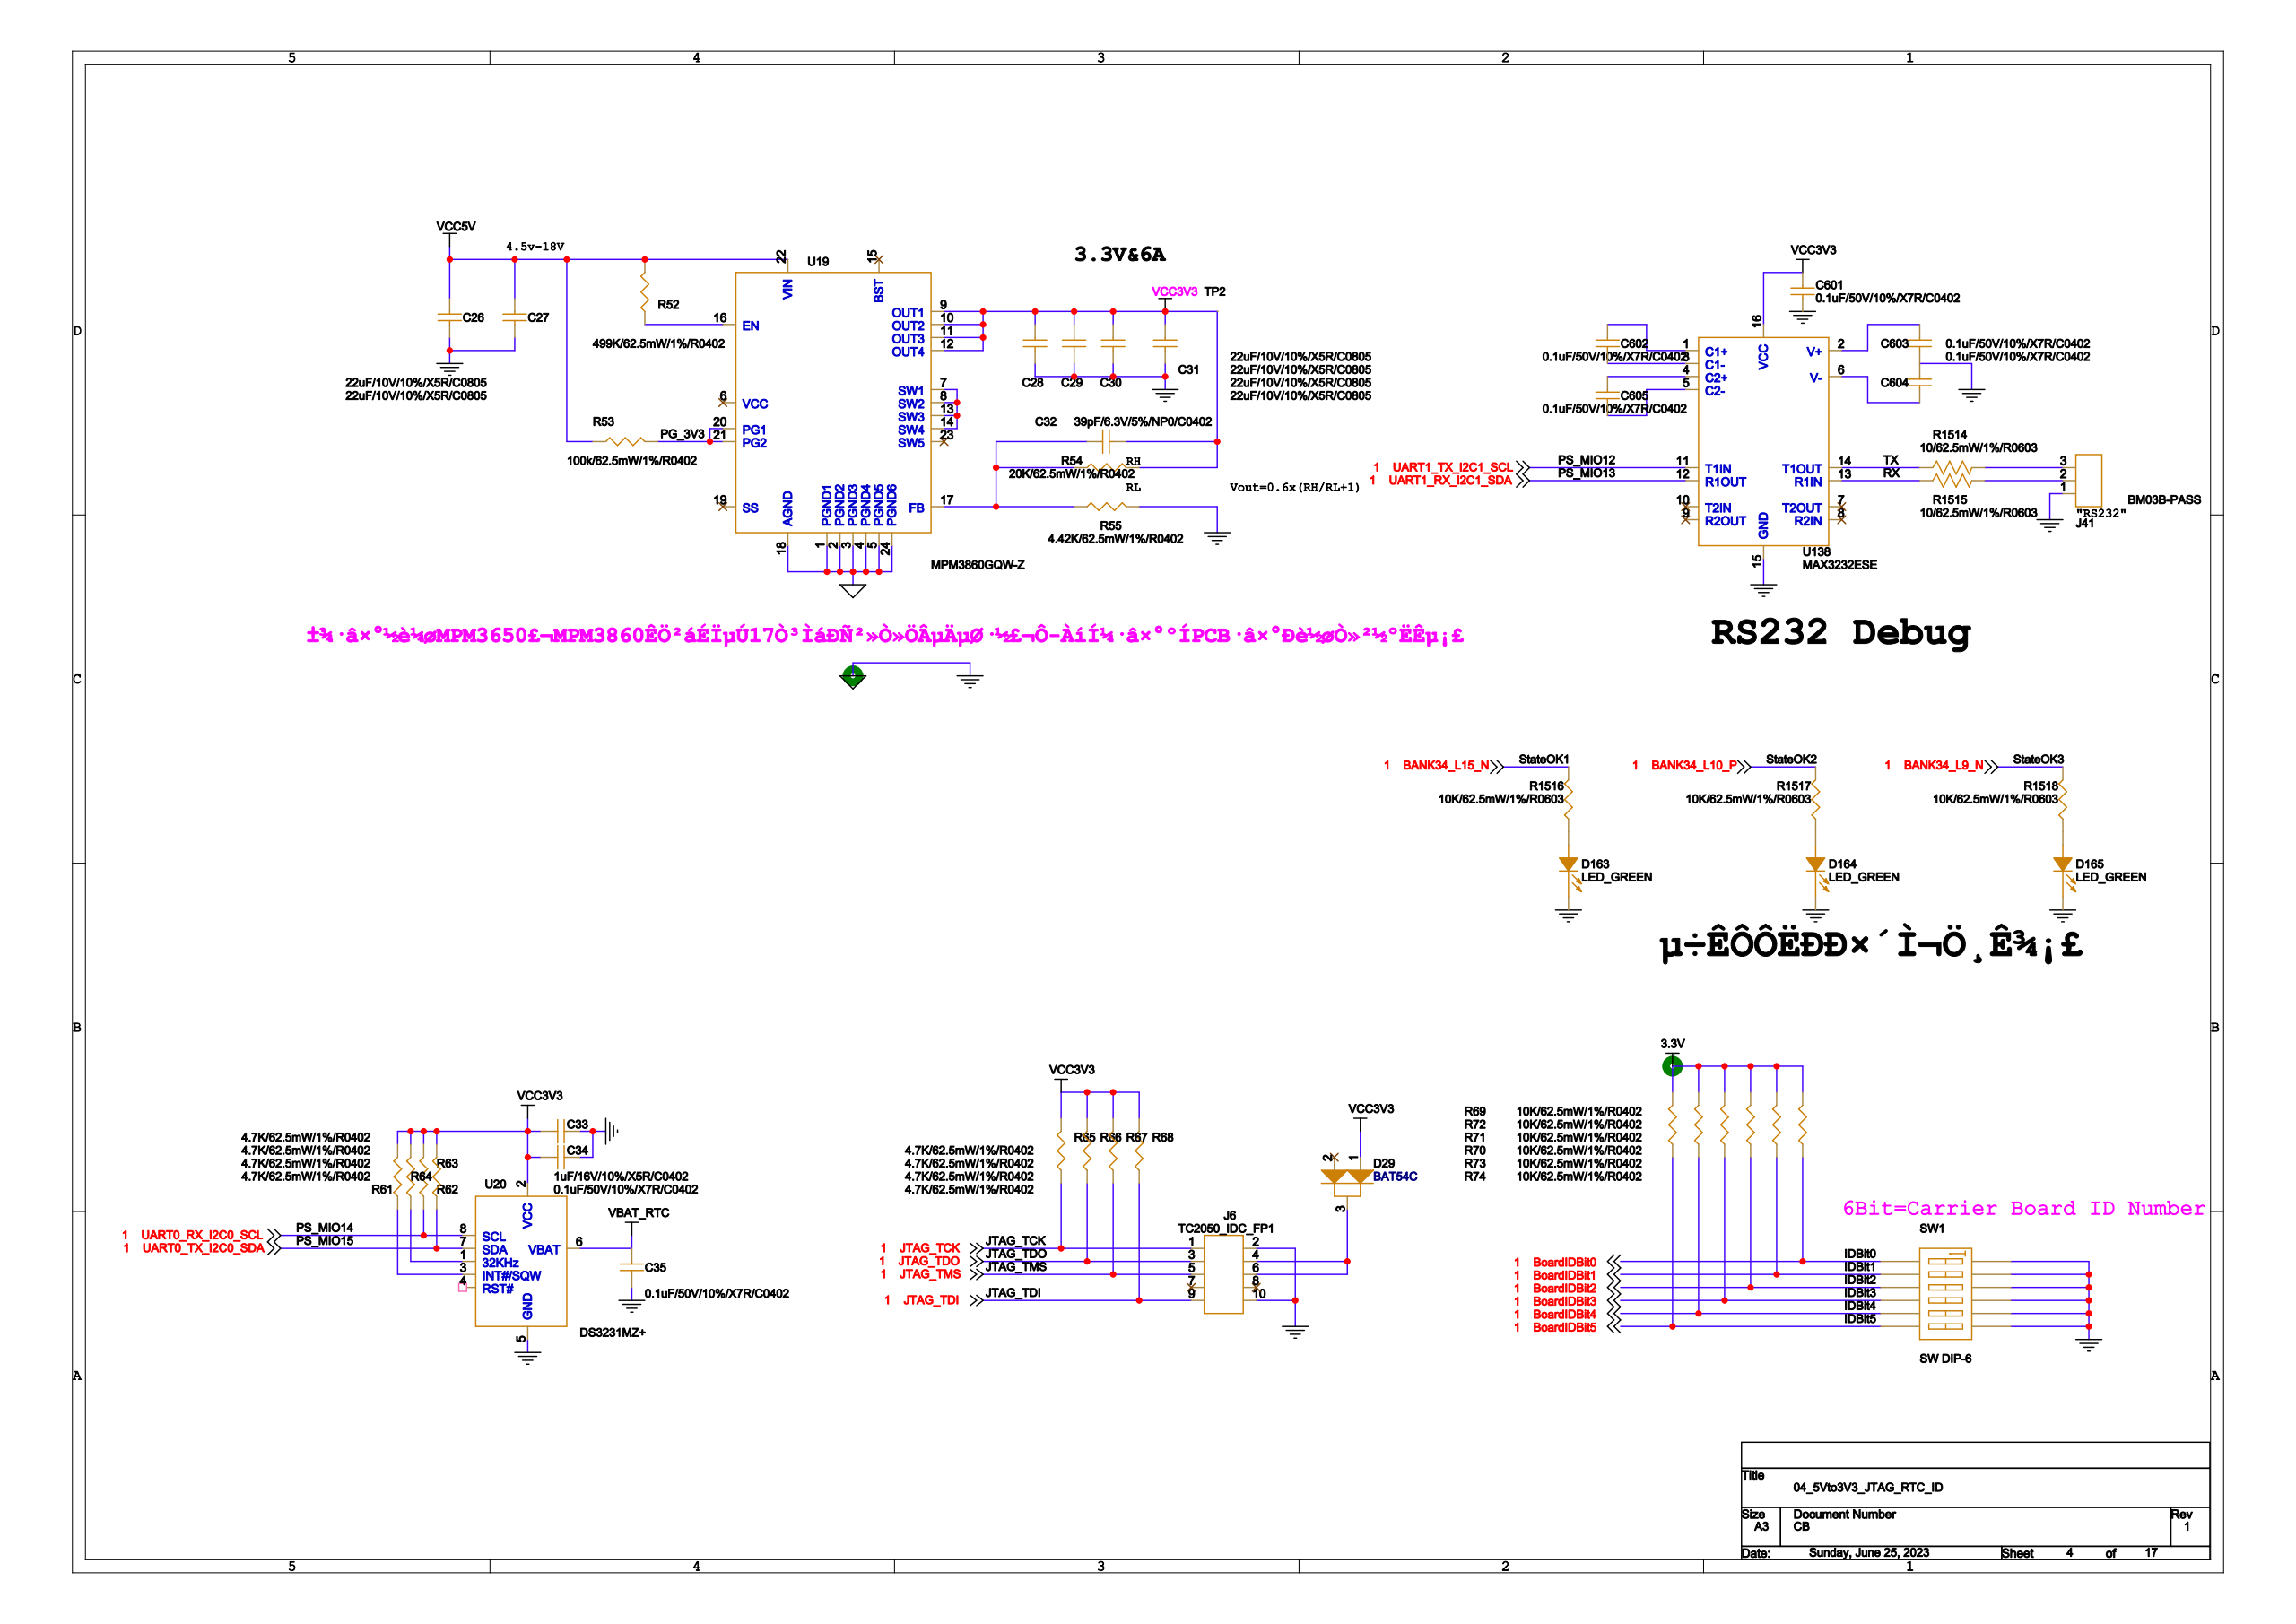Circuit board | Cadence Allegro | 2002 parts | 1538 nets | one sheet of the schematic
Parts on this sheet (reference | value | footprint):
C26 | 22uF/10V/10%/X5R/C0805 | 0805
C27 | 22uF/10V/10%/X5R/C0805 | 0805
C28 | 22uF/10V/10%/X5R/C0805 | 0805
C29 | 22uF/10V/10%/X5R/C0805 | 0805
C30 | 22uF/10V/10%/X5R/C0805 | 0805
C31 | 22uF/10V/10%/X5R/C0805 | 0805
C32 | 39pF/6.3V/5%/NP0/C0402 | 0402
C33 | 1uF/16V/10%/X5R/C0402 | 0402
C34 | 0.1uF/50V/10%/X7R/C0402 | 0402
C35 | 0.1uF/50V/10%/X7R/C0402 | 0402
C601 | 0.1uF/50V/10%/X7R/C0402 | 0402
C602 | 0.1uF/50V/10%/X7R/C0402 | 0402
C603 | 0.1uF/50V/10%/X7R/C0402 | 0402
C604 | 0.1uF/50V/10%/X7R/C0402 | 0402
C605 | 0.1uF/50V/10%/X7R/C0402 | 0402
D29 | BAT54C | SOT23
D163 | LED_GREEN | LED0805
D164 | LED_GREEN | LED0805
D165 | LED_GREEN | LED0805
J6 | TC2050_IDC_FP1 | IDC-TH_Z-231012810106
J41 | BM03B-PASS | BM03B-PASS
R52 | 499K/62.5mW/1%/R0402 | 0402
R53 | 100k/62.5mW/1%/R0402 | 0402
R54 | 20K/62.5mW/1%/R0402 | 0402
R55 | 4.42K/62.5mW/1%/R0402 | 0402
R61 | 4.7K/62.5mW/1%/R0402 | 0402
R62 | 4.7K/62.5mW/1%/R0402 | 0402
R63 | 4.7K/62.5mW/1%/R0402 | 0402
R64 | 4.7K/62.5mW/1%/R0402 | 0402
R65 | 4.7K/62.5mW/1%/R0402 | 0402
R66 | 4.7K/62.5mW/1%/R0402 | 0402
R67 | 4.7K/62.5mW/1%/R0402 | 0402
R68 | 4.7K/62.5mW/1%/R0402 | 0402
R69 | 10K/62.5mW/1%/R0402 | 0402
R70 | 10K/62.5mW/1%/R0402 | 0402
R71 | 10K/62.5mW/1%/R0402 | 0402
R72 | 10K/62.5mW/1%/R0402 | 0402
R73 | 10K/62.5mW/1%/R0402 | 0402
R74 | 10K/62.5mW/1%/R0402 | 0402
R1514 | 10/62.5mW/1%/R0603 | 0603R
R1515 | 10/62.5mW/1%/R0603 | 0603R
R1516 | 10K/62.5mW/1%/R0603 | 0603R
R1517 | 10K/62.5mW/1%/R0603 | 0603R
R1518 | 10K/62.5mW/1%/R0603 | 0603R
SW1 | SW DIP-6 | W-SMD_12P-L9_3-W5_4-P1_27-LS2
TP2 | TEST POINT A | TEST_12MM
U19 | MPM3860GQW-Z | MPM3650GQW
U20 | DS3231MZ+ | SO8
U138 | MAX3232ESE | SO16
Nets of these parts (net: part-pin ...):
3.3V: C28-1 C29-1 C30-1 C31-1 C32-2 C33-2 C34-2 C601-1 D29-1 R54-1 R61-1 R62-1 R63-1 R64-1 R65-1 R66-1 R67-1 R68-1 R69-1 R70-1 R71-1 R72-1 R73-1 R74-1 TP2-1 U19-9 U19-10 U19-11 U19-12 U20-2 U138-16
AGND: C26-2 C27-2 C28-2 C29-2 C30-2 C31-2 C33-1 C34-1 C35-2 C601-2 C603-2 C604-1 D163-2 D164-2 D165-2 J6-2 J6-10 J41-1 R55-1 SW1-7 SW1-8 SW1-9 SW1-10 SW1-11 SW1-12 U19-1 U19-2 U19-3 U19-4 U19-5 U19-18 U19-24 U20-5 U138-15
BOARDIDBIT0: R74-2 SW1-1
BOARDIDBIT1: R73-2 SW1-2
BOARDIDBIT2: R72-2 SW1-3
BOARDIDBIT3: R71-2 SW1-4
BOARDIDBIT4: R70-2 SW1-5
BOARDIDBIT5: R69-2 SW1-6
BANK34_L9_N: R1518-2
BANK34_L10_P: R1517-2
VCC5V: C26-1 C27-1 R52-1 R53-2 U19-22
BANK34_L15_N: R1516-2
JTAG_TDO: J6-3 R66-2
JTAG_TMS: J6-5 R67-2
JTAG_TDI: J6-9 R68-2
JTAG_TCK: J6-1 R65-2
UART0_RX_I2C0_SCL: R63-2 U20-8
UART0_TX_I2C0_SDA: R64-2 U20-7
UART1_TX_I2C1_SCL: U138-11
UART1_RX_I2C1_SDA: U138-12
N23857910: D29-3 J6-4 J6-6
N23931017: J41-2 R1515-2
N23931015: J41-3 R1514-2
N23930865: C602-1 U138-1
N23930898: C602-2 U138-3
N23930926: C605-1 U138-4
N23930940: C605-2 U138-5
RX: R1515-1 U138-13
TX: R1514-1 U138-14
N23930874: C603-1 U138-2
N23930928: C604-2 U138-6
N239315640: D163-1 R1516-1
N239315840: D164-1 R1517-1
N239316020: D165-1 R1518-1
VBAT_RTC: C35-1 U20-6
N23155169: C32-1 R54-2 R55-2 U19-17
N23155064: R52-2 U19-16
PG_3V3: R53-1 U19-20 U19-21
N23857516: R61-2 U20-3
N23857518: R62-2 U20-1
N23155134: U19-7 U19-8 U19-13 U19-14